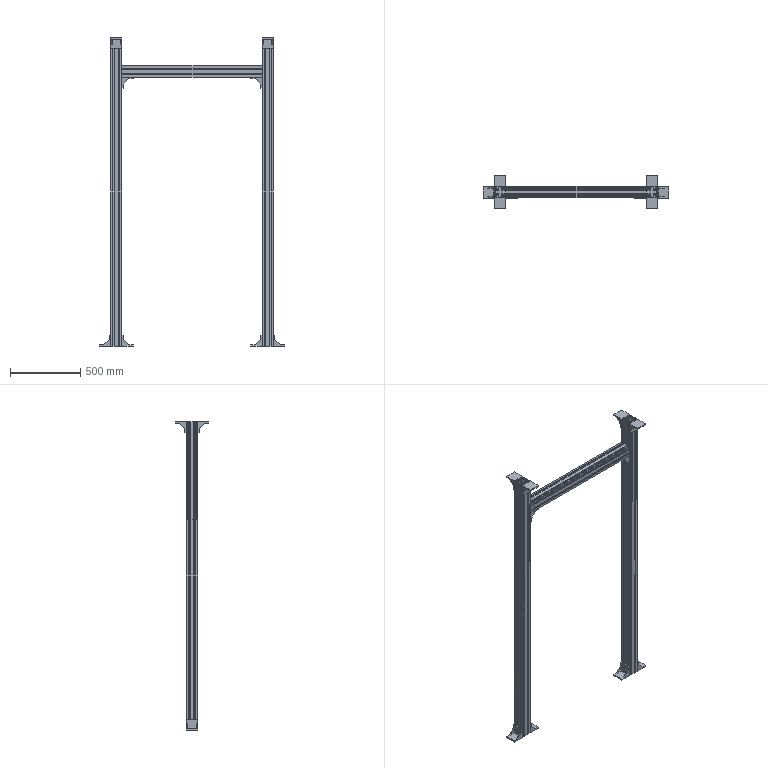Part | NX | features BREP 3 | 13 solids | 528 faces | box 1320 x 240 x 2200 mm | volume 22719197 mm3 | plane 480 | cylinder 48 | commonest cylinder face diameters 6.8 x48